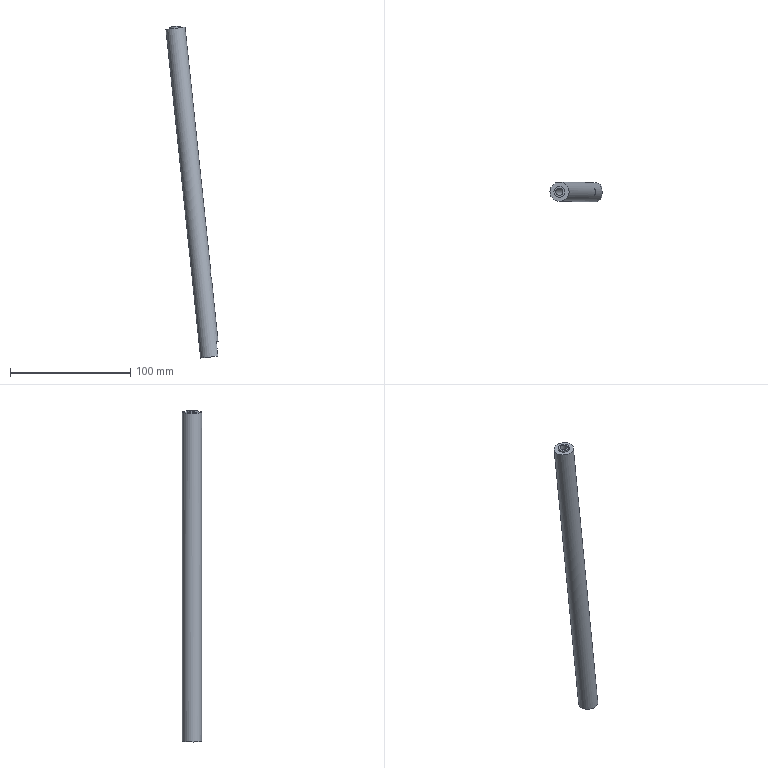Part | STEP file | P011002L002-001 | 1 solid | 20 faces | box 43.362 x 16 x 275.795 mm | volume 48288 mm3 | plane 10 | cylinder 7 | cone 3 | commonest cylinder face diameters 6 x2 6.8 x1 7.973 x1 8 x1 9 x1 16 x1